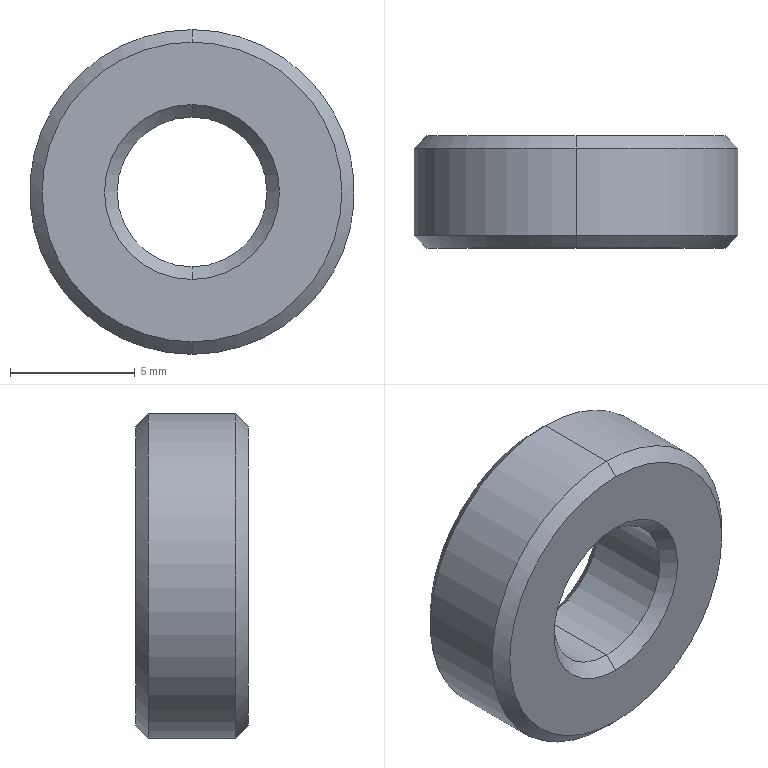Part | SolidWorks | features Chamfer 1, Extrusion 1 | 1 solid | 14 faces | box 13 x 4.5 x 13 mm | volume 455.138 mm3 | cone 8 | cylinder 4 | plane 2 | commonest cylinder face diameters 6 x2 13 x2
STEP:
#1=CARTESIAN_POINT('',(0.,4.5,6.));
#2=VERTEX_POINT('',#1);
#3=CARTESIAN_POINT('',(0.,4.5,-6.));
#4=VERTEX_POINT('',#3);
#5=CARTESIAN_POINT('',(0.,4.5,0.));
#6=DIRECTION('',(0.,1.,0.));
#7=DIRECTION('',(0.,0.,1.));
#8=AXIS2_PLACEMENT_3D('',#5,#6,#7);
#9=CIRCLE('',#8,6.);
#10=EDGE_CURVE('',#2,#4,#9,.T.);
#11=ORIENTED_EDGE('',*,*,#10,.F.);
#12=CARTESIAN_POINT('',(0.,4.,6.5));
#13=VERTEX_POINT('',#12);
#14=CARTESIAN_POINT('',(0.,4.5,6.));
#15=DIRECTION('',(0.,-0.7071,0.7071));
#16=VECTOR('',#15,1000.);
#17=LINE('',#14,#16);
#18=EDGE_CURVE('',#2,#13,#17,.T.);
#19=ORIENTED_EDGE('',*,*,#18,.T.);
#20=CARTESIAN_POINT('',(0.,4.,-6.5));
#21=VERTEX_POINT('',#20);
#22=CARTESIAN_POINT('',(0.,4.,0.));
#23=DIRECTION('',(0.,-1.,0.));
#24=DIRECTION('',(0.,0.,1.));
#25=AXIS2_PLACEMENT_3D('',#22,#23,#24);
#26=CIRCLE('',#25,6.5);
#27=EDGE_CURVE('',#21,#13,#26,.T.);
#28=ORIENTED_EDGE('',*,*,#27,.F.);
#29=CARTESIAN_POINT('',(0.,4.5,-6.));
#30=DIRECTION('',(0.,-0.7071,-0.7071));
#31=VECTOR('',#30,1000.);
#32=LINE('',#29,#31);
#33=EDGE_CURVE('',#4,#21,#32,.T.);
#34=ORIENTED_EDGE('',*,*,#33,.F.);
#35=EDGE_LOOP('',(#11,#19,#28,#34));
#36=FACE_OUTER_BOUND('',#35,.T.);
#37=CARTESIAN_POINT('',(0.,4.5,0.));
#38=DIRECTION('',(0.,-1.,0.));
#39=DIRECTION('',(0.,0.,-1.));
#40=AXIS2_PLACEMENT_3D('',#37,#38,#39);
#41=CONICAL_SURFACE('',#40,6.,0.7854);
#42=ADVANCED_FACE('',(#36),#41,.T.);
#43=CARTESIAN_POINT('',(0.,0.,-6.));
#44=VERTEX_POINT('',#43);
#45=CARTESIAN_POINT('',(0.,0.,6.));
#46=VERTEX_POINT('',#45);
#47=CARTESIAN_POINT('',(0.,0.,0.));
#48=DIRECTION('',(0.,-1.,0.));
#49=DIRECTION('',(0.,0.,1.));
#50=AXIS2_PLACEMENT_3D('',#47,#48,#49);
#51=CIRCLE('',#50,6.);
#52=EDGE_CURVE('',#44,#46,#51,.T.);
#53=ORIENTED_EDGE('',*,*,#52,.F.);
#54=CARTESIAN_POINT('',(0.,0.5,-6.5));
#55=VERTEX_POINT('',#54);
#56=CARTESIAN_POINT('',(0.,0.5,-6.5));
#57=DIRECTION('',(0.,0.7071,-0.7071));
#58=VECTOR('',#57,1000.);
#59=LINE('',#56,#58);
#60=EDGE_CURVE('',#44,#55,#59,.T.);
#61=ORIENTED_EDGE('',*,*,#60,.T.);
#62=CARTESIAN_POINT('',(0.,0.5,6.5));
#63=VERTEX_POINT('',#62);
#64=CARTESIAN_POINT('',(0.,0.5,0.));
#65=DIRECTION('',(0.,1.,0.));
#66=DIRECTION('',(0.,0.,1.));
#67=AXIS2_PLACEMENT_3D('',#64,#65,#66);
#68=CIRCLE('',#67,6.5);
#69=EDGE_CURVE('',#63,#55,#68,.T.);
#70=ORIENTED_EDGE('',*,*,#69,.F.);
#71=CARTESIAN_POINT('',(0.,0.5,6.5));
#72=DIRECTION('',(0.,0.7071,0.7071));
#73=VECTOR('',#72,1000.);
#74=LINE('',#71,#73);
#75=EDGE_CURVE('',#46,#63,#74,.T.);
#76=ORIENTED_EDGE('',*,*,#75,.F.);
#77=EDGE_LOOP('',(#53,#61,#70,#76));
#78=FACE_OUTER_BOUND('',#77,.T.);
#79=CARTESIAN_POINT('',(0.,0.5,0.));
#80=DIRECTION('',(0.,1.,0.));
#81=DIRECTION('',(0.,0.,1.));
#82=AXIS2_PLACEMENT_3D('',#79,#80,#81);
#83=CONICAL_SURFACE('',#82,6.5,0.7854);
#84=ADVANCED_FACE('',(#78),#83,.T.);
#85=CARTESIAN_POINT('',(0.,4.,-3.));
#86=VERTEX_POINT('',#85);
#87=CARTESIAN_POINT('',(0.,4.,3.));
#88=VERTEX_POINT('',#87);
#89=CARTESIAN_POINT('',(0.,4.,0.));
#90=DIRECTION('',(0.,1.,0.));
#91=DIRECTION('',(0.,0.,1.));
#92=AXIS2_PLACEMENT_3D('',#89,#90,#91);
#93=CIRCLE('',#92,3.);
#94=EDGE_CURVE('',#86,#88,#93,.T.);
#95=ORIENTED_EDGE('',*,*,#94,.F.);
#96=CARTESIAN_POINT('',(0.,4.5,-3.5));
#97=VERTEX_POINT('',#96);
#98=CARTESIAN_POINT('',(0.,4.,-3.));
#99=DIRECTION('',(0.,0.7071,-0.7071));
#100=VECTOR('',#99,1000.);
#101=LINE('',#98,#100);
#102=EDGE_CURVE('',#86,#97,#101,.T.);
#103=ORIENTED_EDGE('',*,*,#102,.T.);
#104=CARTESIAN_POINT('',(0.,4.5,3.5));
#105=VERTEX_POINT('',#104);
#106=CARTESIAN_POINT('',(0.,4.5,0.));
#107=DIRECTION('',(0.,-1.,0.));
#108=DIRECTION('',(0.,0.,1.));
#109=AXIS2_PLACEMENT_3D('',#106,#107,#108);
#110=CIRCLE('',#109,3.5);
#111=EDGE_CURVE('',#105,#97,#110,.T.);
#112=ORIENTED_EDGE('',*,*,#111,.F.);
#113=CARTESIAN_POINT('',(0.,4.,3.));
#114=DIRECTION('',(0.,0.7071,0.7071));
#115=VECTOR('',#114,1000.);
#116=LINE('',#113,#115);
#117=EDGE_CURVE('',#88,#105,#116,.T.);
#118=ORIENTED_EDGE('',*,*,#117,.F.);
#119=EDGE_LOOP('',(#95,#103,#112,#118));
#120=FACE_OUTER_BOUND('',#119,.T.);
#121=CARTESIAN_POINT('',(0.,4.,0.));
#122=DIRECTION('',(0.,1.,0.));
#123=DIRECTION('',(0.,0.,1.));
#124=AXIS2_PLACEMENT_3D('',#121,#122,#123);
#125=CONICAL_SURFACE('',#124,3.,0.7854);
#126=ADVANCED_FACE('',(#120),#125,.F.);
#127=CARTESIAN_POINT('',(0.,0.5,3.));
#128=VERTEX_POINT('',#127);
#129=CARTESIAN_POINT('',(0.,0.5,-3.));
#130=VERTEX_POINT('',#129);
#131=CARTESIAN_POINT('',(0.,0.5,0.));
#132=DIRECTION('',(0.,-1.,0.));
#133=DIRECTION('',(0.,0.,1.));
#134=AXIS2_PLACEMENT_3D('',#131,#132,#133);
#135=CIRCLE('',#134,3.);
#136=EDGE_CURVE('',#128,#130,#135,.T.);
#137=ORIENTED_EDGE('',*,*,#136,.F.);
#138=CARTESIAN_POINT('',(0.,0.,3.5));
#139=VERTEX_POINT('',#138);
#140=CARTESIAN_POINT('',(0.,0.,3.5));
#141=DIRECTION('',(0.,-0.7071,0.7071));
#142=VECTOR('',#141,1000.);
#143=LINE('',#140,#142);
#144=EDGE_CURVE('',#128,#139,#143,.T.);
#145=ORIENTED_EDGE('',*,*,#144,.T.);
#146=CARTESIAN_POINT('',(0.,0.,-3.5));
#147=VERTEX_POINT('',#146);
#148=CARTESIAN_POINT('',(0.,0.,0.));
#149=DIRECTION('',(0.,1.,0.));
#150=DIRECTION('',(0.,0.,1.));
#151=AXIS2_PLACEMENT_3D('',#148,#149,#150);
#152=CIRCLE('',#151,3.5);
#153=EDGE_CURVE('',#147,#139,#152,.T.);
#154=ORIENTED_EDGE('',*,*,#153,.F.);
#155=CARTESIAN_POINT('',(0.,0.,-3.5));
#156=DIRECTION('',(0.,-0.7071,-0.7071));
#157=VECTOR('',#156,1000.);
#158=LINE('',#155,#157);
#159=EDGE_CURVE('',#130,#147,#158,.T.);
#160=ORIENTED_EDGE('',*,*,#159,.F.);
#161=EDGE_LOOP('',(#137,#145,#154,#160));
#162=FACE_OUTER_BOUND('',#161,.T.);
#163=CARTESIAN_POINT('',(0.,0.,0.));
#164=DIRECTION('',(0.,-1.,0.));
#165=DIRECTION('',(0.,0.,-1.));
#166=AXIS2_PLACEMENT_3D('',#163,#164,#165);
#167=CONICAL_SURFACE('',#166,3.5,0.7854);
#168=ADVANCED_FACE('',(#162),#167,.F.);
#169=ORIENTED_EDGE('',*,*,#94,.T.);
#170=CARTESIAN_POINT('',(0.,4.5,3.));
#171=DIRECTION('',(0.,-1.,0.));
#172=VECTOR('',#171,1000.);
#173=LINE('',#170,#172);
#174=EDGE_CURVE('',#88,#128,#173,.T.);
#175=ORIENTED_EDGE('',*,*,#174,.T.);
#176=ORIENTED_EDGE('',*,*,#136,.T.);
#177=CARTESIAN_POINT('',(0.,4.5,-3.));
#178=DIRECTION('',(0.,-1.,0.));
#179=VECTOR('',#178,1000.);
#180=LINE('',#177,#179);
#181=EDGE_CURVE('',#86,#130,#180,.T.);
#182=ORIENTED_EDGE('',*,*,#181,.F.);
#183=EDGE_LOOP('',(#169,#175,#176,#182));
#184=FACE_OUTER_BOUND('',#183,.T.);
#185=CARTESIAN_POINT('',(0.,4.5,0.));
#186=DIRECTION('',(0.,-1.,0.));
#187=DIRECTION('',(0.,0.,-1.));
#188=AXIS2_PLACEMENT_3D('',#185,#186,#187);
#189=CYLINDRICAL_SURFACE('',#188,3.);
#190=ADVANCED_FACE('',(#184),#189,.F.);
#191=ORIENTED_EDGE('',*,*,#27,.T.);
#192=CARTESIAN_POINT('',(0.,4.5,6.5));
#193=DIRECTION('',(0.,-1.,0.));
#194=VECTOR('',#193,1000.);
#195=LINE('',#192,#194);
#196=EDGE_CURVE('',#13,#63,#195,.T.);
#197=ORIENTED_EDGE('',*,*,#196,.T.);
#198=ORIENTED_EDGE('',*,*,#69,.T.);
#199=CARTESIAN_POINT('',(0.,4.5,-6.5));
#200=DIRECTION('',(0.,-1.,0.));
#201=VECTOR('',#200,1000.);
#202=LINE('',#199,#201);
#203=EDGE_CURVE('',#21,#55,#202,.T.);
#204=ORIENTED_EDGE('',*,*,#203,.F.);
#205=EDGE_LOOP('',(#191,#197,#198,#204));
#206=FACE_OUTER_BOUND('',#205,.T.);
#207=CARTESIAN_POINT('',(0.,4.5,0.));
#208=DIRECTION('',(0.,-1.,0.));
#209=DIRECTION('',(0.,0.,-1.));
#210=AXIS2_PLACEMENT_3D('',#207,#208,#209);
#211=CYLINDRICAL_SURFACE('',#210,6.5);
#212=ADVANCED_FACE('',(#206),#211,.T.);
#213=ORIENTED_EDGE('',*,*,#111,.T.);
#214=CARTESIAN_POINT('',(0.,4.5,0.));
#215=DIRECTION('',(0.,-1.,0.));
#216=DIRECTION('',(0.,0.,1.));
#217=AXIS2_PLACEMENT_3D('',#214,#215,#216);
#218=CIRCLE('',#217,3.5);
#219=EDGE_CURVE('',#97,#105,#218,.T.);
#220=ORIENTED_EDGE('',*,*,#219,.T.);
#221=EDGE_LOOP('',(#213,#220));
#222=FACE_BOUND('',#221,.T.);
#223=CARTESIAN_POINT('',(0.,4.5,0.));
#224=DIRECTION('',(0.,1.,0.));
#225=DIRECTION('',(0.,0.,1.));
#226=AXIS2_PLACEMENT_3D('',#223,#224,#225);
#227=CIRCLE('',#226,6.);
#228=EDGE_CURVE('',#4,#2,#227,.T.);
#229=ORIENTED_EDGE('',*,*,#228,.T.);
#230=ORIENTED_EDGE('',*,*,#10,.T.);
#231=EDGE_LOOP('',(#229,#230));
#232=FACE_OUTER_BOUND('',#231,.T.);
#233=CARTESIAN_POINT('',(0.,4.5,0.));
#234=DIRECTION('',(0.,1.,0.));
#235=DIRECTION('',(0.,0.,1.));
#236=AXIS2_PLACEMENT_3D('',#233,#234,#235);
#237=PLANE('',#236);
#238=ADVANCED_FACE('',(#222,#232),#237,.T.);
#239=ORIENTED_EDGE('',*,*,#153,.T.);
#240=CARTESIAN_POINT('',(0.,0.,0.));
#241=DIRECTION('',(0.,1.,0.));
#242=DIRECTION('',(0.,0.,1.));
#243=AXIS2_PLACEMENT_3D('',#240,#241,#242);
#244=CIRCLE('',#243,3.5);
#245=EDGE_CURVE('',#139,#147,#244,.T.);
#246=ORIENTED_EDGE('',*,*,#245,.T.);
#247=EDGE_LOOP('',(#239,#246));
#248=FACE_BOUND('',#247,.T.);
#249=CARTESIAN_POINT('',(0.,0.,0.));
#250=DIRECTION('',(0.,-1.,0.));
#251=DIRECTION('',(0.,0.,1.));
#252=AXIS2_PLACEMENT_3D('',#249,#250,#251);
#253=CIRCLE('',#252,6.);
#254=EDGE_CURVE('',#46,#44,#253,.T.);
#255=ORIENTED_EDGE('',*,*,#254,.T.);
#256=ORIENTED_EDGE('',*,*,#52,.T.);
#257=EDGE_LOOP('',(#255,#256));
#258=FACE_OUTER_BOUND('',#257,.T.);
#259=CARTESIAN_POINT('',(0.,0.,0.));
#260=DIRECTION('',(0.,1.,0.));
#261=DIRECTION('',(0.,0.,1.));
#262=AXIS2_PLACEMENT_3D('',#259,#260,#261);
#263=PLANE('',#262);
#264=ADVANCED_FACE('',(#248,#258),#263,.F.);
#265=ORIENTED_EDGE('',*,*,#196,.F.);
#266=CARTESIAN_POINT('',(0.,4.,0.));
#267=DIRECTION('',(0.,-1.,0.));
#268=DIRECTION('',(0.,0.,1.));
#269=AXIS2_PLACEMENT_3D('',#266,#267,#268);
#270=CIRCLE('',#269,6.5);
#271=EDGE_CURVE('',#13,#21,#270,.T.);
#272=ORIENTED_EDGE('',*,*,#271,.T.);
#273=ORIENTED_EDGE('',*,*,#203,.T.);
#274=CARTESIAN_POINT('',(0.,0.5,0.));
#275=DIRECTION('',(0.,1.,0.));
#276=DIRECTION('',(0.,0.,1.));
#277=AXIS2_PLACEMENT_3D('',#274,#275,#276);
#278=CIRCLE('',#277,6.5);
#279=EDGE_CURVE('',#55,#63,#278,.T.);
#280=ORIENTED_EDGE('',*,*,#279,.T.);
#281=EDGE_LOOP('',(#265,#272,#273,#280));
#282=FACE_OUTER_BOUND('',#281,.T.);
#283=CARTESIAN_POINT('',(0.,4.5,0.));
#284=DIRECTION('',(0.,-1.,0.));
#285=DIRECTION('',(0.,0.,-1.));
#286=AXIS2_PLACEMENT_3D('',#283,#284,#285);
#287=CYLINDRICAL_SURFACE('',#286,6.5);
#288=ADVANCED_FACE('',(#282),#287,.T.);
#289=ORIENTED_EDGE('',*,*,#174,.F.);
#290=CARTESIAN_POINT('',(0.,4.,0.));
#291=DIRECTION('',(0.,1.,0.));
#292=DIRECTION('',(0.,0.,1.));
#293=AXIS2_PLACEMENT_3D('',#290,#291,#292);
#294=CIRCLE('',#293,3.);
#295=EDGE_CURVE('',#88,#86,#294,.T.);
#296=ORIENTED_EDGE('',*,*,#295,.T.);
#297=ORIENTED_EDGE('',*,*,#181,.T.);
#298=CARTESIAN_POINT('',(0.,0.5,0.));
#299=DIRECTION('',(0.,-1.,0.));
#300=DIRECTION('',(0.,0.,1.));
#301=AXIS2_PLACEMENT_3D('',#298,#299,#300);
#302=CIRCLE('',#301,3.);
#303=EDGE_CURVE('',#130,#128,#302,.T.);
#304=ORIENTED_EDGE('',*,*,#303,.T.);
#305=EDGE_LOOP('',(#289,#296,#297,#304));
#306=FACE_OUTER_BOUND('',#305,.T.);
#307=CARTESIAN_POINT('',(0.,4.5,0.));
#308=DIRECTION('',(0.,-1.,0.));
#309=DIRECTION('',(0.,0.,-1.));
#310=AXIS2_PLACEMENT_3D('',#307,#308,#309);
#311=CYLINDRICAL_SURFACE('',#310,3.);
#312=ADVANCED_FACE('',(#306),#311,.F.);
#313=ORIENTED_EDGE('',*,*,#144,.F.);
#314=ORIENTED_EDGE('',*,*,#303,.F.);
#315=ORIENTED_EDGE('',*,*,#159,.T.);
#316=ORIENTED_EDGE('',*,*,#245,.F.);
#317=EDGE_LOOP('',(#313,#314,#315,#316));
#318=FACE_OUTER_BOUND('',#317,.T.);
#319=CARTESIAN_POINT('',(0.,0.,0.));
#320=DIRECTION('',(0.,-1.,0.));
#321=DIRECTION('',(0.,0.,-1.));
#322=AXIS2_PLACEMENT_3D('',#319,#320,#321);
#323=CONICAL_SURFACE('',#322,3.5,0.7854);
#324=ADVANCED_FACE('',(#318),#323,.F.);
#325=ORIENTED_EDGE('',*,*,#102,.F.);
#326=ORIENTED_EDGE('',*,*,#295,.F.);
#327=ORIENTED_EDGE('',*,*,#117,.T.);
#328=ORIENTED_EDGE('',*,*,#219,.F.);
#329=EDGE_LOOP('',(#325,#326,#327,#328));
#330=FACE_OUTER_BOUND('',#329,.T.);
#331=CARTESIAN_POINT('',(0.,4.,0.));
#332=DIRECTION('',(0.,1.,0.));
#333=DIRECTION('',(0.,0.,1.));
#334=AXIS2_PLACEMENT_3D('',#331,#332,#333);
#335=CONICAL_SURFACE('',#334,3.,0.7854);
#336=ADVANCED_FACE('',(#330),#335,.F.);
#337=ORIENTED_EDGE('',*,*,#60,.F.);
#338=ORIENTED_EDGE('',*,*,#254,.F.);
#339=ORIENTED_EDGE('',*,*,#75,.T.);
#340=ORIENTED_EDGE('',*,*,#279,.F.);
#341=EDGE_LOOP('',(#337,#338,#339,#340));
#342=FACE_OUTER_BOUND('',#341,.T.);
#343=CARTESIAN_POINT('',(0.,0.5,0.));
#344=DIRECTION('',(0.,1.,0.));
#345=DIRECTION('',(0.,0.,1.));
#346=AXIS2_PLACEMENT_3D('',#343,#344,#345);
#347=CONICAL_SURFACE('',#346,6.5,0.7854);
#348=ADVANCED_FACE('',(#342),#347,.T.);
#349=ORIENTED_EDGE('',*,*,#18,.F.);
#350=ORIENTED_EDGE('',*,*,#228,.F.);
#351=ORIENTED_EDGE('',*,*,#33,.T.);
#352=ORIENTED_EDGE('',*,*,#271,.F.);
#353=EDGE_LOOP('',(#349,#350,#351,#352));
#354=FACE_OUTER_BOUND('',#353,.T.);
#355=CARTESIAN_POINT('',(0.,4.5,0.));
#356=DIRECTION('',(0.,-1.,0.));
#357=DIRECTION('',(0.,0.,-1.));
#358=AXIS2_PLACEMENT_3D('',#355,#356,#357);
#359=CONICAL_SURFACE('',#358,6.,0.7854);
#360=ADVANCED_FACE('',(#354),#359,.T.);
#361=CLOSED_SHELL('',(#42,#84,#126,#168,#190,#212,#238,#264,#288,#312,#324,#336,#348,#360));
#362=MANIFOLD_SOLID_BREP('',#361);
#363=CARTESIAN_POINT('',(0.,0.,0.));
#364=DIRECTION('',(0.,0.,1.));
#365=DIRECTION('',(1.,0.,0.));
#366=AXIS2_PLACEMENT_3D('',#363,#364,#365);
#367=(LENGTH_UNIT()NAMED_UNIT(*)SI_UNIT(.MILLI.,.METRE.));
#368=UNCERTAINTY_MEASURE_WITH_UNIT(LENGTH_MEASURE(0.00001),#367,'','');
#369=(NAMED_UNIT(*)PLANE_ANGLE_UNIT()SI_UNIT($,.RADIAN.));
#370=(NAMED_UNIT(*)SI_UNIT($,.STERADIAN.)SOLID_ANGLE_UNIT());
#371=(GEOMETRIC_REPRESENTATION_CONTEXT(3)GLOBAL_UNCERTAINTY_ASSIGNED_CONTEXT((#368))GLOBAL_UNIT_ASSIGNED_CONTEXT((#367,#369,#370))REPRESENTATION_CONTEXT('',''));
#372=ADVANCED_BREP_SHAPE_REPRESENTATION('',(#362,#366),#371);